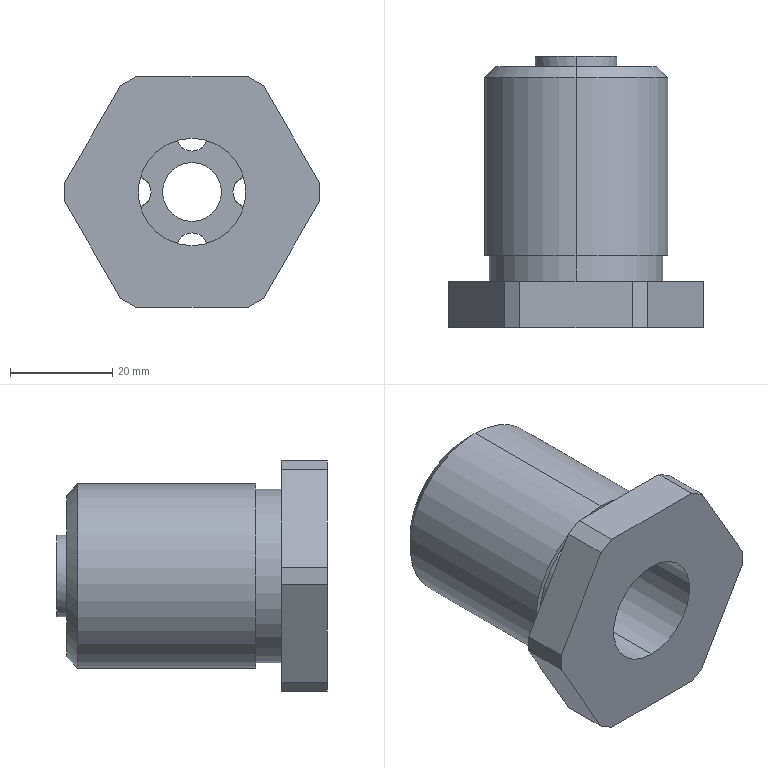Part | SolidWorks | features ICE 8, Chamfer 1, Extrusion 1, HoleWzd 1, StudWizard 1 | 1 solid | 54 faces | box 50 x 53 x 45 mm | volume 40001 mm3 | plane 23 | cylinder 20 | cone 11 | commonest cylinder face diameters 6 x8 11.5 x2 16 x2 21 x2 22 x2 34 x2